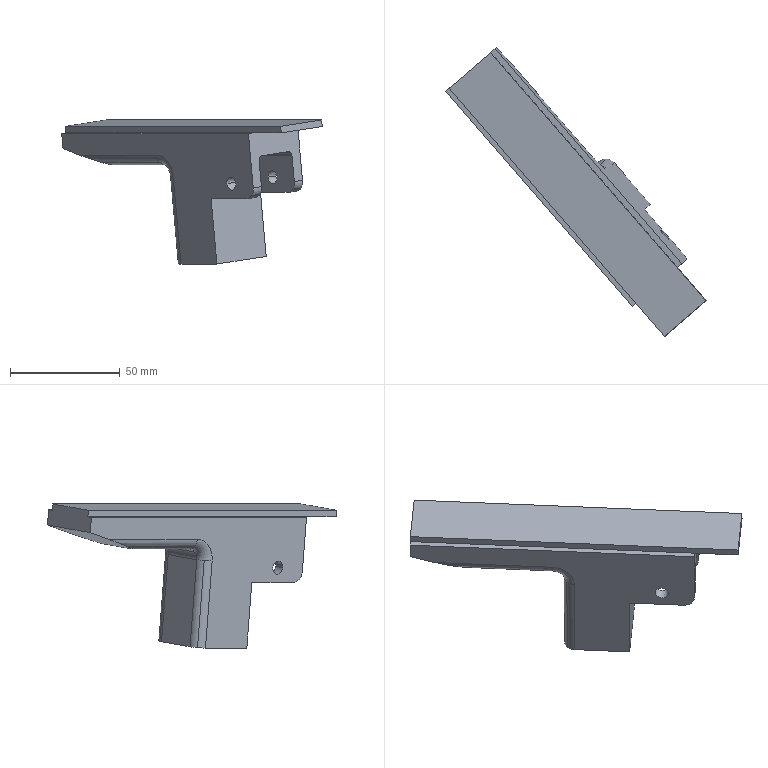Part | SolidWorks | features BaseBody 1 | 1 solid | 45 faces | box 118.942 x 131.952 x 65.78 mm | volume 109548 mm3 | cylinder 22 | plane 21 | torus 2 | commonest cylinder face diameters 10 x14 4 x4 6 x4
STEP:
#1=CARTESIAN_POINT('',(29.752,179.49,-230.441));
#2=VERTEX_POINT('',#1);
#3=CARTESIAN_POINT('',(33.684,174.958,-230.441));
#4=VERTEX_POINT('',#3);
#5=CARTESIAN_POINT('',(31.718,177.224,-230.441));
#6=DIRECTION('',(-0.7501,-0.6509,-0.1168));
#7=DIRECTION('',(0.6554,-0.7553,0.));
#8=AXIS2_PLACEMENT_3D('',#5,#6,#7);
#9=CIRCLE('',#8,3.);
#10=EDGE_CURVE('',#2,#4,#9,.T.);
#11=ORIENTED_EDGE('',*,*,#10,.F.);
#12=CARTESIAN_POINT('',(26.001,176.235,-231.025));
#13=VERTEX_POINT('',#12);
#14=CARTESIAN_POINT('',(48.504,195.763,-227.522));
#15=DIRECTION('',(-0.7501,-0.6509,-0.1168));
#16=VECTOR('',#15,1000.);
#17=LINE('',#14,#16);
#18=EDGE_CURVE('',#2,#13,#17,.T.);
#19=ORIENTED_EDGE('',*,*,#18,.T.);
#20=CARTESIAN_POINT('',(29.934,171.704,-231.025));
#21=VERTEX_POINT('',#20);
#22=CARTESIAN_POINT('',(27.968,173.969,-231.025));
#23=DIRECTION('',(0.7501,0.6509,0.1168));
#24=DIRECTION('',(0.6554,-0.7553,0.));
#25=AXIS2_PLACEMENT_3D('',#22,#23,#24);
#26=CIRCLE('',#25,3.);
#27=EDGE_CURVE('',#21,#13,#26,.T.);
#28=ORIENTED_EDGE('',*,*,#27,.F.);
#29=CARTESIAN_POINT('',(52.437,191.232,-227.522));
#30=DIRECTION('',(-0.7501,-0.6509,-0.1168));
#31=VECTOR('',#30,1000.);
#32=LINE('',#29,#31);
#33=EDGE_CURVE('',#4,#21,#32,.T.);
#34=ORIENTED_EDGE('',*,*,#33,.F.);
#35=EDGE_LOOP('',(#11,#19,#28,#34));
#36=FACE_OUTER_BOUND('',#35,.T.);
#37=CARTESIAN_POINT('',(50.47,193.498,-227.522));
#38=DIRECTION('',(-0.7501,-0.6509,-0.1168));
#39=DIRECTION('',(0.6554,-0.7553,0.));
#40=AXIS2_PLACEMENT_3D('',#37,#38,#39);
#41=CYLINDRICAL_SURFACE('',#40,3.);
#42=ADVANCED_FACE('',(#36),#41,.F.);
#43=CARTESIAN_POINT('',(48.504,195.763,-227.522));
#44=VERTEX_POINT('',#43);
#45=CARTESIAN_POINT('',(52.437,191.232,-227.522));
#46=VERTEX_POINT('',#45);
#47=CARTESIAN_POINT('',(50.47,193.498,-227.522));
#48=DIRECTION('',(-0.7501,-0.6509,-0.1168));
#49=DIRECTION('',(0.6554,-0.7553,0.));
#50=AXIS2_PLACEMENT_3D('',#47,#48,#49);
#51=CIRCLE('',#50,3.);
#52=EDGE_CURVE('',#44,#46,#51,.T.);
#53=ORIENTED_EDGE('',*,*,#52,.F.);
#54=CARTESIAN_POINT('',(44.754,192.509,-228.106));
#55=VERTEX_POINT('',#54);
#56=CARTESIAN_POINT('',(48.504,195.763,-227.522));
#57=DIRECTION('',(-0.7501,-0.6509,-0.1168));
#58=VECTOR('',#57,1000.);
#59=LINE('',#56,#58);
#60=EDGE_CURVE('',#44,#55,#59,.T.);
#61=ORIENTED_EDGE('',*,*,#60,.T.);
#62=CARTESIAN_POINT('',(48.686,187.977,-228.106));
#63=VERTEX_POINT('',#62);
#64=CARTESIAN_POINT('',(46.72,190.243,-228.106));
#65=DIRECTION('',(0.7501,0.6509,0.1168));
#66=DIRECTION('',(0.6554,-0.7553,0.));
#67=AXIS2_PLACEMENT_3D('',#64,#65,#66);
#68=CIRCLE('',#67,3.);
#69=EDGE_CURVE('',#63,#55,#68,.T.);
#70=ORIENTED_EDGE('',*,*,#69,.F.);
#71=CARTESIAN_POINT('',(52.437,191.232,-227.522));
#72=DIRECTION('',(-0.7501,-0.6509,-0.1168));
#73=VECTOR('',#72,1000.);
#74=LINE('',#71,#73);
#75=EDGE_CURVE('',#46,#63,#74,.T.);
#76=ORIENTED_EDGE('',*,*,#75,.F.);
#77=EDGE_LOOP('',(#53,#61,#70,#76));
#78=FACE_OUTER_BOUND('',#77,.T.);
#79=CARTESIAN_POINT('',(50.47,193.498,-227.522));
#80=DIRECTION('',(-0.7501,-0.6509,-0.1168));
#81=DIRECTION('',(0.6554,-0.7553,0.));
#82=AXIS2_PLACEMENT_3D('',#79,#80,#81);
#83=CYLINDRICAL_SURFACE('',#82,3.);
#84=ADVANCED_FACE('',(#78),#83,.F.);
#85=CARTESIAN_POINT('',(-41.121,251.264,-218.114));
#86=VERTEX_POINT('',#85);
#87=CARTESIAN_POINT('',(-31.062,242.523,-221.454));
#88=VERTEX_POINT('',#87);
#89=CARTESIAN_POINT('',(-41.121,251.264,-218.114));
#90=CARTESIAN_POINT('',(-37.715,247.58,-219.449));
#91=CARTESIAN_POINT('',(-34.183,244.51,-220.622));
#92=CARTESIAN_POINT('',(-31.062,242.523,-221.454));
#93=(BOUNDED_CURVE()B_SPLINE_CURVE(3,(#89,#90,#91,#92),.UNSPECIFIED.,.F.,.F.)B_SPLINE_CURVE_WITH_KNOTS((4,4),(4.712,5.498),.UNSPECIFIED.)CURVE()GEOMETRIC_REPRESENTATION_ITEM()RATIONAL_B_SPLINE_CURVE((1.,0.9493,0.9493,1.))REPRESENTATION_ITEM(''));
#94=EDGE_CURVE('',#86,#88,#93,.T.);
#95=ORIENTED_EDGE('',*,*,#94,.T.);
#96=CARTESIAN_POINT('',(-4.54,211.961,-221.454));
#97=VERTEX_POINT('',#96);
#98=CARTESIAN_POINT('',(-9.456,217.625,-221.454));
#99=DIRECTION('',(0.6554,-0.7553,0.));
#100=VECTOR('',#99,1000.);
#101=LINE('',#98,#100);
#102=EDGE_CURVE('',#88,#97,#101,.T.);
#103=ORIENTED_EDGE('',*,*,#102,.T.);
#104=CARTESIAN_POINT('',(-5.95,210.737,-218.114));
#105=VERTEX_POINT('',#104);
#106=CARTESIAN_POINT('',(-2.2,213.992,-217.53));
#107=DIRECTION('',(-0.6554,0.7553,0.));
#108=DIRECTION('',(0.0882,0.07654,-0.9932));
#109=AXIS2_PLACEMENT_3D('',#106,#107,#108);
#110=CIRCLE('',#109,5.);
#111=EDGE_CURVE('',#97,#105,#110,.T.);
#112=ORIENTED_EDGE('',*,*,#111,.T.);
#113=CARTESIAN_POINT('',(-10.866,216.402,-218.114));
#114=DIRECTION('',(-0.6554,0.7553,0.));
#115=VECTOR('',#114,1000.);
#116=LINE('',#113,#115);
#117=EDGE_CURVE('',#105,#86,#116,.T.);
#118=ORIENTED_EDGE('',*,*,#117,.T.);
#119=EDGE_LOOP('',(#95,#103,#112,#118));
#120=FACE_OUTER_BOUND('',#119,.T.);
#121=CARTESIAN_POINT('',(-7.116,219.656,-217.53));
#122=DIRECTION('',(0.6554,-0.7553,0.));
#123=DIRECTION('',(-0.468,-0.4062,-0.7848));
#124=AXIS2_PLACEMENT_3D('',#121,#122,#123);
#125=CYLINDRICAL_SURFACE('',#124,5.);
#126=ADVANCED_FACE('',(#120),#125,.T.);
#127=CARTESIAN_POINT('',(0.2672,207.573,-227.875));
#128=VERTEX_POINT('',#127);
#129=CARTESIAN_POINT('',(1.486,203.95,-228.046));
#130=VERTEX_POINT('',#129);
#131=CARTESIAN_POINT('',(5.236,207.205,-227.462));
#132=DIRECTION('',(-0.0882,-0.07654,0.9932));
#133=DIRECTION('',(-0.6554,0.7553,0.));
#134=AXIS2_PLACEMENT_3D('',#131,#132,#133);
#135=CIRCLE('',#134,5.);
#136=EDGE_CURVE('',#128,#130,#135,.T.);
#137=ORIENTED_EDGE('',*,*,#136,.F.);
#138=CARTESIAN_POINT('',(3.795,210.635,-267.601));
#139=VERTEX_POINT('',#138);
#140=CARTESIAN_POINT('',(-0.1738,207.191,-222.909));
#141=DIRECTION('',(0.0882,0.07654,-0.9932));
#142=VECTOR('',#141,1000.);
#143=LINE('',#140,#142);
#144=EDGE_CURVE('',#128,#139,#143,.T.);
#145=ORIENTED_EDGE('',*,*,#144,.T.);
#146=CARTESIAN_POINT('',(5.014,207.011,-267.772));
#147=VERTEX_POINT('',#146);
#148=CARTESIAN_POINT('',(8.764,210.266,-267.188));
#149=DIRECTION('',(-0.0882,-0.07654,0.9932));
#150=DIRECTION('',(-0.9939,0.07376,-0.08257));
#151=AXIS2_PLACEMENT_3D('',#148,#149,#150);
#152=CIRCLE('',#151,5.);
#153=EDGE_CURVE('',#139,#147,#152,.T.);
#154=ORIENTED_EDGE('',*,*,#153,.T.);
#155=CARTESIAN_POINT('',(1.045,203.567,-223.08));
#156=DIRECTION('',(-0.0882,-0.07654,0.9932));
#157=VECTOR('',#156,1000.);
#158=LINE('',#155,#157);
#159=EDGE_CURVE('',#147,#130,#158,.T.);
#160=ORIENTED_EDGE('',*,*,#159,.T.);
#161=EDGE_LOOP('',(#137,#145,#154,#160));
#162=FACE_OUTER_BOUND('',#161,.T.);
#163=CARTESIAN_POINT('',(4.795,206.822,-222.496));
#164=DIRECTION('',(0.0882,0.07654,-0.9932));
#165=DIRECTION('',(-0.9939,0.07376,-0.08257));
#166=AXIS2_PLACEMENT_3D('',#163,#164,#165);
#167=CYLINDRICAL_SURFACE('',#166,5.);
#168=ADVANCED_FACE('',(#162),#167,.T.);
#169=CARTESIAN_POINT('',(15.689,224.835,-221.615));
#170=VERTEX_POINT('',#169);
#171=CARTESIAN_POINT('',(13.243,227.393,-220.16));
#172=VERTEX_POINT('',#171);
#173=CARTESIAN_POINT('',(13.684,227.776,-225.126));
#174=DIRECTION('',(-0.7501,-0.6509,-0.1168));
#175=DIRECTION('',(0.4011,-0.5882,0.7023));
#176=AXIS2_PLACEMENT_3D('',#173,#174,#175);
#177=CIRCLE('',#176,5.);
#178=EDGE_CURVE('',#170,#172,#177,.T.);
#179=ORIENTED_EDGE('',*,*,#178,.F.);
#180=CARTESIAN_POINT('',(0.6876,211.816,-223.95));
#181=VERTEX_POINT('',#180);
#182=CARTESIAN_POINT('',(19.44,228.09,-221.031));
#183=DIRECTION('',(-0.7501,-0.6509,-0.1168));
#184=VECTOR('',#183,1000.);
#185=LINE('',#182,#184);
#186=EDGE_CURVE('',#170,#181,#185,.T.);
#187=ORIENTED_EDGE('',*,*,#186,.T.);
#188=CARTESIAN_POINT('',(-1.759,214.375,-222.496));
#189=VERTEX_POINT('',#188);
#190=CARTESIAN_POINT('',(-1.318,214.757,-227.462));
#191=DIRECTION('',(0.7501,0.6509,0.1168));
#192=DIRECTION('',(0.4011,-0.5882,0.7023));
#193=AXIS2_PLACEMENT_3D('',#190,#191,#192);
#194=CIRCLE('',#193,5.);
#195=EDGE_CURVE('',#189,#181,#194,.T.);
#196=ORIENTED_EDGE('',*,*,#195,.F.);
#197=CARTESIAN_POINT('',(16.993,230.648,-219.577));
#198=DIRECTION('',(0.7501,0.6509,0.1168));
#199=VECTOR('',#198,1000.);
#200=LINE('',#197,#199);
#201=EDGE_CURVE('',#189,#172,#200,.T.);
#202=ORIENTED_EDGE('',*,*,#201,.T.);
#203=EDGE_LOOP('',(#179,#187,#196,#202));
#204=FACE_OUTER_BOUND('',#203,.T.);
#205=CARTESIAN_POINT('',(17.434,231.031,-224.542));
#206=DIRECTION('',(-0.7501,-0.6509,-0.1168));
#207=DIRECTION('',(0.4011,-0.5882,0.7023));
#208=AXIS2_PLACEMENT_3D('',#205,#206,#207);
#209=CYLINDRICAL_SURFACE('',#208,5.);
#210=ADVANCED_FACE('',(#204),#209,.F.);
#211=CARTESIAN_POINT('',(-9.697,253.827,-220.16));
#212=VERTEX_POINT('',#211);
#213=CARTESIAN_POINT('',(-10.756,260.145,-218.293));
#214=VERTEX_POINT('',#213);
#215=CARTESIAN_POINT('',(-9.697,253.827,-220.16));
#216=CARTESIAN_POINT('',(-8.689,254.702,-220.004));
#217=CARTESIAN_POINT('',(-9.061,256.92,-219.348));
#218=CARTESIAN_POINT('',(-10.756,260.145,-218.293));
#219=(BOUNDED_CURVE()B_SPLINE_CURVE(3,(#215,#216,#217,#218),.UNSPECIFIED.,.F.,.F.)B_SPLINE_CURVE_WITH_KNOTS((4,4),(0.,0.7854),.UNSPECIFIED.)CURVE()GEOMETRIC_REPRESENTATION_ITEM()RATIONAL_B_SPLINE_CURVE((1.,0.9493,0.9493,1.))REPRESENTATION_ITEM(''));
#220=EDGE_CURVE('',#212,#214,#219,.T.);
#221=ORIENTED_EDGE('',*,*,#220,.T.);
#222=CARTESIAN_POINT('',(15.766,229.583,-218.293));
#223=VERTEX_POINT('',#222);
#224=CARTESIAN_POINT('',(10.85,235.247,-218.293));
#225=DIRECTION('',(0.6554,-0.7553,0.));
#226=VECTOR('',#225,1000.);
#227=LINE('',#224,#226);
#228=EDGE_CURVE('',#214,#223,#227,.T.);
#229=ORIENTED_EDGE('',*,*,#228,.T.);
#230=CARTESIAN_POINT('',(12.802,227.011,-215.195));
#231=DIRECTION('',(-0.6554,0.7553,0.));
#232=DIRECTION('',(0.7501,0.6509,0.1168));
#233=AXIS2_PLACEMENT_3D('',#230,#231,#232);
#234=CIRCLE('',#233,5.);
#235=EDGE_CURVE('',#223,#172,#234,.T.);
#236=ORIENTED_EDGE('',*,*,#235,.T.);
#237=CARTESIAN_POINT('',(8.327,233.058,-220.16));
#238=DIRECTION('',(-0.6554,0.7553,0.));
#239=VECTOR('',#238,1000.);
#240=LINE('',#237,#239);
#241=EDGE_CURVE('',#172,#212,#240,.T.);
#242=ORIENTED_EDGE('',*,*,#241,.T.);
#243=EDGE_LOOP('',(#221,#229,#236,#242));
#244=FACE_OUTER_BOUND('',#243,.T.);
#245=CARTESIAN_POINT('',(7.886,232.675,-215.195));
#246=DIRECTION('',(0.6554,-0.7553,0.));
#247=DIRECTION('',(0.5928,0.5144,-0.6197));
#248=AXIS2_PLACEMENT_3D('',#245,#246,#247);
#249=CYLINDRICAL_SURFACE('',#248,5.);
#250=ADVANCED_FACE('',(#244),#249,.T.);
#251=CARTESIAN_POINT('',(20.573,225.195,-224.713));
#252=VERTEX_POINT('',#251);
#253=CARTESIAN_POINT('',(16.961,224.,-225.126));
#254=VERTEX_POINT('',#253);
#255=CARTESIAN_POINT('',(20.238,220.224,-225.126));
#256=DIRECTION('',(-0.0882,-0.07654,0.9932));
#257=DIRECTION('',(0.7501,0.6509,0.1168));
#258=AXIS2_PLACEMENT_3D('',#255,#256,#257);
#259=CIRCLE('',#258,5.);
#260=EDGE_CURVE('',#252,#254,#259,.T.);
#261=ORIENTED_EDGE('',*,*,#260,.F.);
#262=CARTESIAN_POINT('',(24.101,228.257,-264.44));
#263=VERTEX_POINT('',#262);
#264=CARTESIAN_POINT('',(20.132,224.813,-219.748));
#265=DIRECTION('',(0.0882,0.07654,-0.9932));
#266=VECTOR('',#265,1000.);
#267=LINE('',#264,#266);
#268=EDGE_CURVE('',#252,#263,#267,.T.);
#269=ORIENTED_EDGE('',*,*,#268,.T.);
#270=CARTESIAN_POINT('',(20.489,227.061,-264.853));
#271=VERTEX_POINT('',#270);
#272=CARTESIAN_POINT('',(23.766,223.285,-264.853));
#273=DIRECTION('',(-0.0882,-0.07654,0.9932));
#274=DIRECTION('',(0.06694,0.9943,0.08257));
#275=AXIS2_PLACEMENT_3D('',#272,#273,#274);
#276=CIRCLE('',#275,5.);
#277=EDGE_CURVE('',#263,#271,#276,.T.);
#278=ORIENTED_EDGE('',*,*,#277,.T.);
#279=CARTESIAN_POINT('',(16.52,223.617,-220.16));
#280=DIRECTION('',(-0.0882,-0.07654,0.9932));
#281=VECTOR('',#280,1000.);
#282=LINE('',#279,#281);
#283=EDGE_CURVE('',#271,#254,#282,.T.);
#284=ORIENTED_EDGE('',*,*,#283,.T.);
#285=EDGE_LOOP('',(#261,#269,#278,#284));
#286=FACE_OUTER_BOUND('',#285,.T.);
#287=CARTESIAN_POINT('',(19.797,219.841,-220.16));
#288=DIRECTION('',(0.0882,0.07654,-0.9932));
#289=DIRECTION('',(0.06694,0.9943,0.08257));
#290=AXIS2_PLACEMENT_3D('',#287,#288,#289);
#291=CYLINDRICAL_SURFACE('',#290,5.);
#292=ADVANCED_FACE('',(#286),#291,.T.);
#293=CARTESIAN_POINT('',(55.669,178.149,-218.174));
#294=VERTEX_POINT('',#293);
#295=CARTESIAN_POINT('',(55.105,177.659,-216.838));
#296=VERTEX_POINT('',#295);
#297=CARTESIAN_POINT('',(54.169,176.847,-218.408));
#298=DIRECTION('',(0.6554,-0.7553,0.));
#299=DIRECTION('',(0.468,0.4062,0.7848));
#300=AXIS2_PLACEMENT_3D('',#297,#298,#299);
#301=CIRCLE('',#300,2.);
#302=EDGE_CURVE('',#294,#296,#301,.T.);
#303=ORIENTED_EDGE('',*,*,#302,.T.);
#304=CARTESIAN_POINT('',(38.72,196.541,-216.838));
#305=VERTEX_POINT('',#304);
#306=CARTESIAN_POINT('',(55.105,177.659,-216.838));
#307=DIRECTION('',(-0.6554,0.7553,0.));
#308=VECTOR('',#307,1000.);
#309=LINE('',#306,#308);
#310=EDGE_CURVE('',#296,#305,#309,.T.);
#311=ORIENTED_EDGE('',*,*,#310,.T.);
#312=CARTESIAN_POINT('',(39.284,197.03,-218.174));
#313=VERTEX_POINT('',#312);
#314=CARTESIAN_POINT('',(37.784,195.728,-218.408));
#315=DIRECTION('',(0.6554,-0.7553,0.));
#316=DIRECTION('',(0.468,0.4062,0.7848));
#317=AXIS2_PLACEMENT_3D('',#314,#315,#316);
#318=CIRCLE('',#317,2.);
#319=EDGE_CURVE('',#313,#305,#318,.T.);
#320=ORIENTED_EDGE('',*,*,#319,.F.);
#321=CARTESIAN_POINT('',(55.669,178.149,-218.174));
#322=DIRECTION('',(0.6554,-0.7553,0.));
#323=VECTOR('',#322,1000.);
#324=LINE('',#321,#323);
#325=EDGE_CURVE('',#313,#294,#324,.T.);
#326=ORIENTED_EDGE('',*,*,#325,.T.);
#327=EDGE_LOOP('',(#303,#311,#320,#326));
#328=FACE_OUTER_BOUND('',#327,.T.);
#329=CARTESIAN_POINT('',(54.169,176.847,-218.408));
#330=DIRECTION('',(-0.6554,0.7553,0.));
#331=DIRECTION('',(0.468,0.4062,0.7848));
#332=AXIS2_PLACEMENT_3D('',#329,#330,#331);
#333=CYLINDRICAL_SURFACE('',#332,2.);
#334=ADVANCED_FACE('',(#328),#333,.F.);
#335=CARTESIAN_POINT('',(41.991,166.279,-218.29));
#336=VERTEX_POINT('',#335);
#337=CARTESIAN_POINT('',(40.982,165.403,-219.037));
#338=VERTEX_POINT('',#337);
#339=CARTESIAN_POINT('',(42.168,166.432,-220.276));
#340=DIRECTION('',(0.6554,-0.7553,0.));
#341=DIRECTION('',(-0.5928,-0.5144,0.6197));
#342=AXIS2_PLACEMENT_3D('',#339,#340,#341);
#343=CIRCLE('',#342,2.);
#344=EDGE_CURVE('',#336,#338,#343,.T.);
#345=ORIENTED_EDGE('',*,*,#344,.T.);
#346=CARTESIAN_POINT('',(24.597,184.284,-219.037));
#347=VERTEX_POINT('',#346);
#348=CARTESIAN_POINT('',(40.982,165.403,-219.037));
#349=DIRECTION('',(-0.6554,0.7553,0.));
#350=VECTOR('',#349,1000.);
#351=LINE('',#348,#350);
#352=EDGE_CURVE('',#338,#347,#351,.T.);
#353=ORIENTED_EDGE('',*,*,#352,.T.);
#354=CARTESIAN_POINT('',(25.606,185.16,-218.29));
#355=VERTEX_POINT('',#354);
#356=CARTESIAN_POINT('',(25.782,185.313,-220.276));
#357=DIRECTION('',(0.6554,-0.7553,0.));
#358=DIRECTION('',(-0.5928,-0.5144,0.6197));
#359=AXIS2_PLACEMENT_3D('',#356,#357,#358);
#360=CIRCLE('',#359,2.);
#361=EDGE_CURVE('',#355,#347,#360,.T.);
#362=ORIENTED_EDGE('',*,*,#361,.F.);
#363=CARTESIAN_POINT('',(41.991,166.279,-218.29));
#364=DIRECTION('',(0.6554,-0.7553,0.));
#365=VECTOR('',#364,1000.);
#366=LINE('',#363,#365);
#367=EDGE_CURVE('',#355,#336,#366,.T.);
#368=ORIENTED_EDGE('',*,*,#367,.T.);
#369=EDGE_LOOP('',(#345,#353,#362,#368));
#370=FACE_OUTER_BOUND('',#369,.T.);
#371=CARTESIAN_POINT('',(42.168,166.432,-220.276));
#372=DIRECTION('',(-0.6554,0.7553,0.));
#373=DIRECTION('',(-0.5928,-0.5144,0.6197));
#374=AXIS2_PLACEMENT_3D('',#371,#372,#373);
#375=CYLINDRICAL_SURFACE('',#374,2.);
#376=ADVANCED_FACE('',(#370),#375,.F.);
#377=CARTESIAN_POINT('',(37.976,162.794,-233.011));
#378=VERTEX_POINT('',#377);
#379=CARTESIAN_POINT('',(37.328,164.17,-236.523));
#380=VERTEX_POINT('',#379);
#381=CARTESIAN_POINT('',(34.698,166.57,-233.011));
#382=DIRECTION('',(0.7501,0.6509,0.1168));
#383=DIRECTION('',(0.5258,-0.4799,-0.7023));
#384=AXIS2_PLACEMENT_3D('',#381,#382,#383);
#385=CIRCLE('',#384,5.);
#386=EDGE_CURVE('',#378,#380,#385,.T.);
#387=ORIENTED_EDGE('',*,*,#386,.T.);
#388=CARTESIAN_POINT('',(41.078,167.425,-235.939));
#389=VERTEX_POINT('',#388);
#390=CARTESIAN_POINT('',(37.328,164.17,-236.523));
#391=DIRECTION('',(0.7501,0.6509,0.1168));
#392=VECTOR('',#391,1000.);
#393=LINE('',#390,#392);
#394=EDGE_CURVE('',#380,#389,#393,.T.);
#395=ORIENTED_EDGE('',*,*,#394,.T.);
#396=CARTESIAN_POINT('',(41.726,166.048,-232.428));
#397=VERTEX_POINT('',#396);
#398=CARTESIAN_POINT('',(38.449,169.825,-232.428));
#399=DIRECTION('',(-0.7501,-0.6509,-0.1168));
#400=DIRECTION('',(0.5258,-0.4799,-0.7023));
#401=AXIS2_PLACEMENT_3D('',#398,#399,#400);
#402=CIRCLE('',#401,5.);
#403=EDGE_CURVE('',#389,#397,#402,.T.);
#404=ORIENTED_EDGE('',*,*,#403,.T.);
#405=CARTESIAN_POINT('',(37.976,162.794,-233.011));
#406=DIRECTION('',(-0.7501,-0.6509,-0.1168));
#407=VECTOR('',#406,1000.);
#408=LINE('',#405,#407);
#409=EDGE_CURVE('',#397,#378,#408,.T.);
#410=ORIENTED_EDGE('',*,*,#409,.T.);
#411=EDGE_LOOP('',(#387,#395,#404,#410));
#412=FACE_OUTER_BOUND('',#411,.T.);
#413=CARTESIAN_POINT('',(34.698,166.57,-233.011));
#414=DIRECTION('',(0.7501,0.6509,0.1168));
#415=DIRECTION('',(0.5258,-0.4799,-0.7023));
#416=AXIS2_PLACEMENT_3D('',#413,#414,#415);
#417=CYLINDRICAL_SURFACE('',#416,5.);
#418=ADVANCED_FACE('',(#412),#417,.T.);
#419=CARTESIAN_POINT('',(56.728,179.067,-230.092));
#420=VERTEX_POINT('',#419);
#421=CARTESIAN_POINT('',(56.08,180.444,-233.603));
#422=VERTEX_POINT('',#421);
#423=CARTESIAN_POINT('',(53.451,182.843,-230.092));
#424=DIRECTION('',(0.7501,0.6509,0.1168));
#425=DIRECTION('',(0.5258,-0.4799,-0.7023));
#426=AXIS2_PLACEMENT_3D('',#423,#424,#425);
#427=CIRCLE('',#426,5.);
#428=EDGE_CURVE('',#420,#422,#427,.T.);
#429=ORIENTED_EDGE('',*,*,#428,.T.);
#430=CARTESIAN_POINT('',(59.83,183.698,-233.02));
#431=VERTEX_POINT('',#430);
#432=CARTESIAN_POINT('',(37.328,164.17,-236.523));
#433=DIRECTION('',(0.7501,0.6509,0.1168));
#434=VECTOR('',#433,1000.);
#435=LINE('',#432,#434);
#436=EDGE_CURVE('',#422,#431,#435,.T.);
#437=ORIENTED_EDGE('',*,*,#436,.T.);
#438=CARTESIAN_POINT('',(60.478,182.322,-229.508));
#439=VERTEX_POINT('',#438);
#440=CARTESIAN_POINT('',(57.201,186.098,-229.508));
#441=DIRECTION('',(-0.7501,-0.6509,-0.1168));
#442=DIRECTION('',(0.5258,-0.4799,-0.7023));
#443=AXIS2_PLACEMENT_3D('',#440,#441,#442);
#444=CIRCLE('',#443,5.);
#445=EDGE_CURVE('',#431,#439,#444,.T.);
#446=ORIENTED_EDGE('',*,*,#445,.T.);
#447=CARTESIAN_POINT('',(37.976,162.794,-233.011));
#448=DIRECTION('',(-0.7501,-0.6509,-0.1168));
#449=VECTOR('',#448,1000.);
#450=LINE('',#447,#449);
#451=EDGE_CURVE('',#439,#420,#450,.T.);
#452=ORIENTED_EDGE('',*,*,#451,.T.);
#453=EDGE_LOOP('',(#429,#437,#446,#452));
#454=FACE_OUTER_BOUND('',#453,.T.);
#455=CARTESIAN_POINT('',(34.698,166.57,-233.011));
#456=DIRECTION('',(0.7501,0.6509,0.1168));
#457=DIRECTION('',(0.5258,-0.4799,-0.7023));
#458=AXIS2_PLACEMENT_3D('',#455,#456,#457);
#459=CYLINDRICAL_SURFACE('',#458,5.);
#460=ADVANCED_FACE('',(#454),#459,.T.);
#461=ORIENTED_EDGE('',*,*,#27,.T.);
#462=CARTESIAN_POINT('',(27.968,173.969,-231.025));
#463=DIRECTION('',(0.7501,0.6509,0.1168));
#464=DIRECTION('',(0.6554,-0.7553,0.));
#465=AXIS2_PLACEMENT_3D('',#462,#463,#464);
#466=CIRCLE('',#465,3.);
#467=EDGE_CURVE('',#13,#21,#466,.T.);
#468=ORIENTED_EDGE('',*,*,#467,.T.);
#469=EDGE_LOOP('',(#461,#468));
#470=FACE_BOUND('',#469,.T.);
#471=ORIENTED_EDGE('',*,*,#159,.F.);
#472=CARTESIAN_POINT('',(21.4,188.13,-267.772));
#473=VERTEX_POINT('',#472);
#474=CARTESIAN_POINT('',(1.737,210.788,-267.772));
#475=DIRECTION('',(0.6554,-0.7553,0.));
#476=VECTOR('',#475,1000.);
#477=LINE('',#474,#476);
#478=EDGE_CURVE('',#147,#473,#477,.T.);
#479=ORIENTED_EDGE('',*,*,#478,.T.);
#480=CARTESIAN_POINT('',(18.754,185.834,-237.977));
#481=VERTEX_POINT('',#480);
#482=CARTESIAN_POINT('',(21.4,188.13,-267.772));
#483=DIRECTION('',(-0.0882,-0.07654,0.9932));
#484=VECTOR('',#483,1000.);
#485=LINE('',#482,#484);
#486=EDGE_CURVE('',#473,#481,#485,.T.);
#487=ORIENTED_EDGE('',*,*,#486,.T.);
#488=CARTESIAN_POINT('',(35.139,166.952,-237.977));
#489=VERTEX_POINT('',#488);
#490=CARTESIAN_POINT('',(38.417,163.176,-237.977));
#491=DIRECTION('',(-0.6554,0.7553,0.));
#492=VECTOR('',#491,1000.);
#493=LINE('',#490,#492);
#494=EDGE_CURVE('',#489,#481,#493,.T.);
#495=ORIENTED_EDGE('',*,*,#494,.F.);
#496=CARTESIAN_POINT('',(34.698,166.57,-233.011));
#497=DIRECTION('',(0.7501,0.6509,0.1168));
#498=DIRECTION('',(0.5258,-0.4799,-0.7023));
#499=AXIS2_PLACEMENT_3D('',#496,#497,#498);
#500=CIRCLE('',#499,5.);
#501=EDGE_CURVE('',#380,#489,#500,.T.);
#502=ORIENTED_EDGE('',*,*,#501,.F.);
#503=ORIENTED_EDGE('',*,*,#386,.F.);
#504=CARTESIAN_POINT('',(35.771,160.88,-208.183));
#505=VERTEX_POINT('',#504);
#506=CARTESIAN_POINT('',(35.771,160.88,-208.183));
#507=DIRECTION('',(0.0882,0.07654,-0.9932));
#508=VECTOR('',#507,1000.);
#509=LINE('',#506,#508);
#510=EDGE_CURVE('',#505,#378,#509,.T.);
#511=ORIENTED_EDGE('',*,*,#510,.F.);
#512=CARTESIAN_POINT('',(-49.435,259.063,-208.183));
#513=VERTEX_POINT('',#512);
#514=CARTESIAN_POINT('',(16.108,183.538,-208.183));
#515=DIRECTION('',(-0.6554,0.7553,0.));
#516=VECTOR('',#515,1000.);
#517=LINE('',#514,#516);
#518=EDGE_CURVE('',#505,#513,#517,.T.);
#519=ORIENTED_EDGE('',*,*,#518,.T.);
#520=CARTESIAN_POINT('',(-48.821,259.596,-215.096));
#521=VERTEX_POINT('',#520);
#522=CARTESIAN_POINT('',(-49.435,259.063,-208.183));
#523=DIRECTION('',(0.0882,0.07654,-0.9932));
#524=VECTOR('',#523,1000.);
#525=LINE('',#522,#524);
#526=EDGE_CURVE('',#513,#521,#525,.T.);
#527=ORIENTED_EDGE('',*,*,#526,.T.);
#528=CARTESIAN_POINT('',(-6.615,213.929,-231.636));
#529=DIRECTION('',(-0.6559,0.7097,0.257));
#530=VECTOR('',#529,1000.);
#531=LINE('',#528,#530);
#532=EDGE_CURVE('',#86,#521,#531,.T.);
#533=ORIENTED_EDGE('',*,*,#532,.F.);
#534=ORIENTED_EDGE('',*,*,#117,.F.);
#535=CARTESIAN_POINT('',(-5.068,211.503,-228.046));
#536=DIRECTION('',(-0.7501,-0.6509,-0.1168));
#537=DIRECTION('',(0.4011,-0.5882,0.7023));
#538=AXIS2_PLACEMENT_3D('',#535,#536,#537);
#539=CIRCLE('',#538,10.);
#540=EDGE_CURVE('',#130,#105,#539,.T.);
#541=ORIENTED_EDGE('',*,*,#540,.F.);
#542=EDGE_LOOP('',(#471,#479,#487,#495,#502,#503,#511,#519,#527,#533,#534,#541));
#543=FACE_OUTER_BOUND('',#542,.T.);
#544=CARTESIAN_POINT('',(27.262,173.357,-223.08));
#545=DIRECTION('',(0.7501,0.6509,0.1168));
#546=DIRECTION('',(-0.6554,0.7553,0.));
#547=AXIS2_PLACEMENT_3D('',#544,#545,#546);
#548=PLANE('',#547);
#549=ADVANCED_FACE('',(#470,#543),#548,.F.);
#550=ORIENTED_EDGE('',*,*,#409,.F.);
#551=CARTESIAN_POINT('',(40.668,165.13,-220.51));
#552=VERTEX_POINT('',#551);
#553=CARTESIAN_POINT('',(40.997,165.415,-224.213));
#554=DIRECTION('',(-0.0882,-0.07654,0.9932));
#555=VECTOR('',#554,1000.);
#556=LINE('',#553,#555);
#557=EDGE_CURVE('',#397,#552,#556,.T.);
#558=ORIENTED_EDGE('',*,*,#557,.T.);
#559=CARTESIAN_POINT('',(42.168,166.432,-220.276));
#560=DIRECTION('',(0.6554,-0.7553,0.));
#561=DIRECTION('',(-0.5928,-0.5144,0.6197));
#562=AXIS2_PLACEMENT_3D('',#559,#560,#561);
#563=CIRCLE('',#562,2.);
#564=EDGE_CURVE('',#338,#552,#563,.T.);
#565=ORIENTED_EDGE('',*,*,#564,.F.);
#566=ORIENTED_EDGE('',*,*,#344,.F.);
#567=CARTESIAN_POINT('',(53.993,176.694,-216.421));
#568=VERTEX_POINT('',#567);
#569=CARTESIAN_POINT('',(38.616,163.349,-218.815));
#570=DIRECTION('',(0.7501,0.6509,0.1168));
#571=VECTOR('',#570,1000.);
#572=LINE('',#569,#571);
#573=EDGE_CURVE('',#336,#568,#572,.T.);
#574=ORIENTED_EDGE('',*,*,#573,.T.);
#575=CARTESIAN_POINT('',(54.169,176.847,-218.408));
#576=DIRECTION('',(0.6554,-0.7553,0.));
#577=DIRECTION('',(0.468,0.4062,0.7848));
#578=AXIS2_PLACEMENT_3D('',#575,#576,#577);
#579=CIRCLE('',#578,2.);
#580=EDGE_CURVE('',#296,#568,#579,.T.);
#581=ORIENTED_EDGE('',*,*,#580,.F.);
#582=ORIENTED_EDGE('',*,*,#302,.F.);
#583=CARTESIAN_POINT('',(55.008,177.575,-210.725));
#584=DIRECTION('',(0.0882,0.07654,-0.9932));
#585=VECTOR('',#584,1000.);
#586=LINE('',#583,#585);
#587=EDGE_CURVE('',#294,#420,#586,.T.);
#588=ORIENTED_EDGE('',*,*,#587,.T.);
#589=ORIENTED_EDGE('',*,*,#451,.F.);
#590=CARTESIAN_POINT('',(58.273,180.408,-204.679));
#591=VERTEX_POINT('',#590);
#592=CARTESIAN_POINT('',(58.273,180.408,-204.679));
#593=DIRECTION('',(0.0882,0.07654,-0.9932));
#594=VECTOR('',#593,1000.);
#595=LINE('',#592,#594);
#596=EDGE_CURVE('',#591,#439,#595,.T.);
#597=ORIENTED_EDGE('',*,*,#596,.F.);
#598=CARTESIAN_POINT('',(56.398,178.781,-204.971));
#599=VERTEX_POINT('',#598);
#600=CARTESIAN_POINT('',(35.771,160.88,-208.183));
#601=DIRECTION('',(0.7501,0.6509,0.1168));
#602=VECTOR('',#601,1000.);
#603=LINE('',#600,#602);
#604=EDGE_CURVE('',#599,#591,#603,.T.);
#605=ORIENTED_EDGE('',*,*,#604,.F.);
#606=CARTESIAN_POINT('',(37.646,162.507,-207.891));
#607=VERTEX_POINT('',#606);
#608=CARTESIAN_POINT('',(35.771,160.88,-208.183));
#609=DIRECTION('',(0.7501,0.6509,0.1168));
#610=VECTOR('',#609,1000.);
#611=LINE('',#608,#610);
#612=EDGE_CURVE('',#607,#599,#611,.T.);
#613=ORIENTED_EDGE('',*,*,#612,.F.);
#614=CARTESIAN_POINT('',(35.771,160.88,-208.183));
#615=DIRECTION('',(0.7501,0.6509,0.1168));
#616=VECTOR('',#615,1000.);
#617=LINE('',#614,#616);
#618=EDGE_CURVE('',#505,#607,#617,.T.);
#619=ORIENTED_EDGE('',*,*,#618,.F.);
#620=ORIENTED_EDGE('',*,*,#510,.T.);
#621=EDGE_LOOP('',(#550,#558,#565,#566,#574,#581,#582,#588,#589,#597,#605,#613,#619,#620));
#622=FACE_OUTER_BOUND('',#621,.T.);
#623=CARTESIAN_POINT('',(35.771,160.88,-208.183));
#624=DIRECTION('',(0.6554,-0.7553,0.));
#625=DIRECTION('',(-0.0882,-0.07654,0.9932));
#626=AXIS2_PLACEMENT_3D('',#623,#624,#625);
#627=PLANE('',#626);
#628=ADVANCED_FACE('',(#622),#627,.T.);
#629=CARTESIAN_POINT('',(37.607,195.575,-216.421));
#630=VERTEX_POINT('',#629);
#631=CARTESIAN_POINT('',(53.993,176.694,-216.421));
#632=DIRECTION('',(-0.6554,0.7553,0.));
#633=VECTOR('',#632,1000.);
#634=LINE('',#631,#633);
#635=EDGE_CURVE('',#568,#630,#634,.T.);
#636=ORIENTED_EDGE('',*,*,#635,.F.);
#637=ORIENTED_EDGE('',*,*,#573,.F.);
#638=ORIENTED_EDGE('',*,*,#367,.F.);
#639=CARTESIAN_POINT('',(24.106,183.858,-218.523));
#640=DIRECTION('',(0.7501,0.6509,0.1168));
#641=VECTOR('',#640,1000.);
#642=LINE('',#639,#641);
#643=EDGE_CURVE('',#355,#630,#642,.T.);
#644=ORIENTED_EDGE('',*,*,#643,.T.);
#645=EDGE_LOOP('',(#636,#637,#638,#644));
#646=FACE_OUTER_BOUND('',#645,.T.);
#647=CARTESIAN_POINT('',(40.491,164.977,-218.523));
#648=DIRECTION('',(-0.0882,-0.07654,0.9932));
#649=DIRECTION('',(-0.6554,0.7553,0.));
#650=AXIS2_PLACEMENT_3D('',#647,#648,#649);
#651=PLANE('',#650);
#652=ADVANCED_FACE('',(#646),#651,.F.);
#653=ORIENTED_EDGE('',*,*,#436,.F.);
#654=CARTESIAN_POINT('',(53.892,183.226,-235.058));
#655=VERTEX_POINT('',#654);
#656=CARTESIAN_POINT('',(53.451,182.843,-230.092));
#657=DIRECTION('',(0.7501,0.6509,0.1168));
#658=DIRECTION('',(0.5258,-0.4799,-0.7023));
#659=AXIS2_PLACEMENT_3D('',#656,#657,#658);
#660=CIRCLE('',#659,5.);
#661=EDGE_CURVE('',#422,#655,#660,.T.);
#662=ORIENTED_EDGE('',*,*,#661,.T.);
#663=CARTESIAN_POINT('',(57.642,186.481,-234.474));
#664=VERTEX_POINT('',#663);
#665=CARTESIAN_POINT('',(35.139,166.952,-237.977));
#666=DIRECTION('',(0.7501,0.6509,0.1168));
#667=VECTOR('',#666,1000.);
#668=LINE('',#665,#667);
#669=EDGE_CURVE('',#655,#664,#668,.T.);
#670=ORIENTED_EDGE('',*,*,#669,.T.);
#671=CARTESIAN_POINT('',(57.201,186.098,-229.508));
#672=DIRECTION('',(-0.7501,-0.6509,-0.1168));
#673=DIRECTION('',(0.5258,-0.4799,-0.7023));
#674=AXIS2_PLACEMENT_3D('',#671,#672,#673);
#675=CIRCLE('',#674,5.);
#676=EDGE_CURVE('',#664,#431,#675,.T.);
#677=ORIENTED_EDGE('',*,*,#676,.T.);
#678=EDGE_LOOP('',(#653,#662,#670,#677));
#679=FACE_OUTER_BOUND('',#678,.T.);
#680=CARTESIAN_POINT('',(34.698,166.57,-233.011));
#681=DIRECTION('',(0.7501,0.6509,0.1168));
#682=DIRECTION('',(0.5258,-0.4799,-0.7023));
#683=AXIS2_PLACEMENT_3D('',#680,#681,#682);
#684=CYLINDRICAL_SURFACE('',#683,5.);
#685=ADVANCED_FACE('',(#679),#684,.T.);
#686=CARTESIAN_POINT('',(38.89,170.207,-237.393));
#687=VERTEX_POINT('',#686);
#688=CARTESIAN_POINT('',(35.139,166.952,-237.977));
#689=DIRECTION('',(0.7501,0.6509,0.1168));
#690=VECTOR('',#689,1000.);
#691=LINE('',#688,#690);
#692=EDGE_CURVE('',#489,#687,#691,.T.);
#693=ORIENTED_EDGE('',*,*,#692,.F.);
#694=ORIENTED_EDGE('',*,*,#494,.T.);
#695=CARTESIAN_POINT('',(41.256,205.362,-234.474));
#696=VERTEX_POINT('',#695);
#697=CARTESIAN_POINT('',(18.754,185.834,-237.977));
#698=DIRECTION('',(0.7501,0.6509,0.1168));
#699=VECTOR('',#698,1000.);
#700=LINE('',#697,#699);
#701=EDGE_CURVE('',#481,#696,#700,.T.);
#702=ORIENTED_EDGE('',*,*,#701,.T.);
#703=CARTESIAN_POINT('',(60.919,182.705,-234.474));
#704=DIRECTION('',(-0.6554,0.7553,0.));
#705=VECTOR('',#704,1000.);
#706=LINE('',#703,#705);
#707=EDGE_CURVE('',#664,#696,#706,.T.);
#708=ORIENTED_EDGE('',*,*,#707,.F.);
#709=ORIENTED_EDGE('',*,*,#669,.F.);
#710=CARTESIAN_POINT('',(40.783,198.331,-235.058));
#711=VERTEX_POINT('',#710);
#712=CARTESIAN_POINT('',(57.169,179.45,-235.058));
#713=DIRECTION('',(-0.6554,0.7553,0.));
#714=VECTOR('',#713,1000.);
#715=LINE('',#712,#714);
#716=EDGE_CURVE('',#655,#711,#715,.T.);
#717=ORIENTED_EDGE('',*,*,#716,.T.);
#718=CARTESIAN_POINT('',(25.781,185.312,-237.393));
#719=VERTEX_POINT('',#718);
#720=CARTESIAN_POINT('',(27.656,186.94,-237.101));
#721=DIRECTION('',(-0.7501,-0.6509,-0.1168));
#722=VECTOR('',#721,1000.);
#723=LINE('',#720,#722);
#724=EDGE_CURVE('',#711,#719,#723,.T.);
#725=ORIENTED_EDGE('',*,*,#724,.T.);
#726=CARTESIAN_POINT('',(42.167,166.431,-237.393));
#727=DIRECTION('',(0.6554,-0.7553,0.));
#728=VECTOR('',#727,1000.);
#729=LINE('',#726,#728);
#730=EDGE_CURVE('',#719,#687,#729,.T.);
#731=ORIENTED_EDGE('',*,*,#730,.T.);
#732=EDGE_LOOP('',(#693,#694,#702,#708,#709,#717,#725,#731));
#733=FACE_OUTER_BOUND('',#732,.T.);
#734=CARTESIAN_POINT('',(38.417,163.176,-237.977));
#735=DIRECTION('',(0.0882,0.07654,-0.9932));
#736=DIRECTION('',(-0.7501,-0.6509,-0.1168));
#737=AXIS2_PLACEMENT_3D('',#734,#735,#736);
#738=PLANE('',#737);
#739=ADVANCED_FACE('',(#733),#738,.T.);
#740=ORIENTED_EDGE('',*,*,#394,.F.);
#741=ORIENTED_EDGE('',*,*,#501,.T.);
#742=ORIENTED_EDGE('',*,*,#692,.T.);
#743=CARTESIAN_POINT('',(38.449,169.825,-232.428));
#744=DIRECTION('',(-0.7501,-0.6509,-0.1168));
#745=DIRECTION('',(0.5258,-0.4799,-0.7023));
#746=AXIS2_PLACEMENT_3D('',#743,#744,#745);
#747=CIRCLE('',#746,5.);
#748=EDGE_CURVE('',#687,#389,#747,.T.);
#749=ORIENTED_EDGE('',*,*,#748,.T.);
#750=EDGE_LOOP('',(#740,#741,#742,#749));
#751=FACE_OUTER_BOUND('',#750,.T.);
#752=CARTESIAN_POINT('',(34.698,166.57,-233.011));
#753=DIRECTION('',(0.7501,0.6509,0.1168));
#754=DIRECTION('',(0.5258,-0.4799,-0.7023));
#755=AXIS2_PLACEMENT_3D('',#752,#753,#754);
#756=CYLINDRICAL_SURFACE('',#755,5.);
#757=ADVANCED_FACE('',(#751),#756,.T.);
#758=CARTESIAN_POINT('',(31.718,177.224,-230.441));
#759=DIRECTION('',(-0.7501,-0.6509,-0.1168));
#760=DIRECTION('',(0.6554,-0.7553,0.));
#761=AXIS2_PLACEMENT_3D('',#758,#759,#760);
#762=CIRCLE('',#761,3.);
#763=EDGE_CURVE('',#4,#2,#762,.T.);
#764=ORIENTED_EDGE('',*,*,#763,.T.);
#765=ORIENTED_EDGE('',*,*,#10,.T.);
#766=EDGE_LOOP('',(#764,#765));
#767=FACE_BOUND('',#766,.T.);
#768=CARTESIAN_POINT('',(24.282,184.011,-220.51));
#769=VERTEX_POINT('',#768);
#770=CARTESIAN_POINT('',(40.668,165.13,-220.51));
#771=DIRECTION('',(-0.6554,0.7553,0.));
#772=VECTOR('',#771,1000.);
#773=LINE('',#770,#772);
#774=EDGE_CURVE('',#552,#769,#773,.T.);
#775=ORIENTED_EDGE('',*,*,#774,.F.);
#776=ORIENTED_EDGE('',*,*,#557,.F.);
#777=ORIENTED_EDGE('',*,*,#403,.F.);
#778=ORIENTED_EDGE('',*,*,#748,.F.);
#779=ORIENTED_EDGE('',*,*,#730,.F.);
#780=CARTESIAN_POINT('',(26.086,185.577,-240.827));
#781=DIRECTION('',(-0.0882,-0.07654,0.9932));
#782=VECTOR('',#781,1000.);
#783=LINE('',#780,#782);
#784=EDGE_CURVE('',#719,#769,#783,.T.);
#785=ORIENTED_EDGE('',*,*,#784,.T.);
#786=EDGE_LOOP('',(#775,#776,#777,#778,#779,#785));
#787=FACE_OUTER_BOUND('',#786,.T.);
#788=CARTESIAN_POINT('',(42.472,166.696,-240.827));
#789=DIRECTION('',(-0.7501,-0.6509,-0.1168));
#790=DIRECTION('',(0.0882,0.07654,-0.9932));
#791=AXIS2_PLACEMENT_3D('',#788,#789,#790);
#792=PLANE('',#791);
#793=ADVANCED_FACE('',(#767,#787),#792,.F.);
#794=ORIENTED_EDGE('',*,*,#319,.T.);
#795=CARTESIAN_POINT('',(37.784,195.728,-218.408));
#796=DIRECTION('',(0.6554,-0.7553,0.));
#797=DIRECTION('',(0.468,0.4062,0.7848));
#798=AXIS2_PLACEMENT_3D('',#795,#796,#797);
#799=CIRCLE('',#798,2.);
#800=EDGE_CURVE('',#305,#630,#799,.T.);
#801=ORIENTED_EDGE('',*,*,#800,.T.);
#802=ORIENTED_EDGE('',*,*,#643,.F.);
#803=ORIENTED_EDGE('',*,*,#361,.T.);
#804=CARTESIAN_POINT('',(25.782,185.313,-220.276));
#805=DIRECTION('',(0.6554,-0.7553,0.));
#806=DIRECTION('',(-0.5928,-0.5144,0.6197));
#807=AXIS2_PLACEMENT_3D('',#804,#805,#806);
#808=CIRCLE('',#807,2.);
#809=EDGE_CURVE('',#347,#769,#808,.T.);
#810=ORIENTED_EDGE('',*,*,#809,.T.);
#811=ORIENTED_EDGE('',*,*,#784,.F.);
#812=ORIENTED_EDGE('',*,*,#724,.F.);
#813=CARTESIAN_POINT('',(39.107,196.877,-216.188));
#814=DIRECTION('',(0.0882,0.07654,-0.9932));
#815=VECTOR('',#814,1000.);
#816=LINE('',#813,#815);
#817=EDGE_CURVE('',#313,#711,#816,.T.);
#818=ORIENTED_EDGE('',*,*,#817,.F.);
#819=EDGE_LOOP('',(#794,#801,#802,#803,#810,#811,#812,#818));
#820=FACE_OUTER_BOUND('',#819,.T.);
#821=CARTESIAN_POINT('',(32.597,191.227,-228.507));
#822=DIRECTION('',(-0.6554,0.7553,0.));
#823=DIRECTION('',(-0.0882,-0.07654,0.9932));
#824=AXIS2_PLACEMENT_3D('',#821,#822,#823);
#825=PLANE('',#824);
#826=ADVANCED_FACE('',(#820),#825,.F.);
#827=ORIENTED_EDGE('',*,*,#352,.F.);
#828=ORIENTED_EDGE('',*,*,#564,.T.);
#829=ORIENTED_EDGE('',*,*,#774,.T.);
#830=ORIENTED_EDGE('',*,*,#809,.F.);
#831=EDGE_LOOP('',(#827,#828,#829,#830));
#832=FACE_OUTER_BOUND('',#831,.T.);
#833=CARTESIAN_POINT('',(42.168,166.432,-220.276));
#834=DIRECTION('',(-0.6554,0.7553,0.));
#835=DIRECTION('',(-0.5928,-0.5144,0.6197));
#836=AXIS2_PLACEMENT_3D('',#833,#834,#835);
#837=CYLINDRICAL_SURFACE('',#836,2.);
#838=ADVANCED_FACE('',(#832),#837,.F.);
#839=ORIENTED_EDGE('',*,*,#69,.T.);
#840=CARTESIAN_POINT('',(46.72,190.243,-228.106));
#841=DIRECTION('',(0.7501,0.6509,0.1168));
#842=DIRECTION('',(0.6554,-0.7553,0.));
#843=AXIS2_PLACEMENT_3D('',#840,#841,#842);
#844=CIRCLE('',#843,3.);
#845=EDGE_CURVE('',#55,#63,#844,.T.);
#846=ORIENTED_EDGE('',*,*,#845,.T.);
#847=EDGE_LOOP('',(#839,#846));
#848=FACE_BOUND('',#847,.T.);
#849=ORIENTED_EDGE('',*,*,#325,.F.);
#850=ORIENTED_EDGE('',*,*,#817,.T.);
#851=ORIENTED_EDGE('',*,*,#716,.F.);
#852=ORIENTED_EDGE('',*,*,#661,.F.);
#853=ORIENTED_EDGE('',*,*,#428,.F.);
#854=ORIENTED_EDGE('',*,*,#587,.F.);
#855=EDGE_LOOP('',(#849,#850,#851,#852,#853,#854));
#856=FACE_OUTER_BOUND('',#855,.T.);
#857=CARTESIAN_POINT('',(55.493,177.996,-216.188));
#858=DIRECTION('',(0.7501,0.6509,0.1168));
#859=DIRECTION('',(-0.6554,0.7553,0.));
#860=AXIS2_PLACEMENT_3D('',#857,#858,#859);
#861=PLANE('',#860);
#862=ADVANCED_FACE('',(#848,#856),#861,.F.);
#863=ORIENTED_EDGE('',*,*,#310,.F.);
#864=ORIENTED_EDGE('',*,*,#580,.T.);
#865=ORIENTED_EDGE('',*,*,#635,.T.);
#866=ORIENTED_EDGE('',*,*,#800,.F.);
#867=EDGE_LOOP('',(#863,#864,#865,#866));
#868=FACE_OUTER_BOUND('',#867,.T.);
#869=CARTESIAN_POINT('',(54.169,176.847,-218.408));
#870=DIRECTION('',(-0.6554,0.7553,0.));
#871=DIRECTION('',(0.468,0.4062,0.7848));
#872=AXIS2_PLACEMENT_3D('',#869,#870,#871);
#873=CYLINDRICAL_SURFACE('',#872,2.);
#874=ADVANCED_FACE('',(#868),#873,.F.);
#875=CARTESIAN_POINT('',(-47.56,260.691,-207.891));
#876=VERTEX_POINT('',#875);
#877=CARTESIAN_POINT('',(50.754,147.402,-207.891));
#878=DIRECTION('',(-0.6554,0.7553,0.));
#879=VECTOR('',#878,1000.);
#880=LINE('',#877,#879);
#881=EDGE_CURVE('',#607,#876,#880,.T.);
#882=ORIENTED_EDGE('',*,*,#881,.T.);
#883=CARTESIAN_POINT('',(-26.932,278.592,-204.679));
#884=DIRECTION('',(-0.7501,-0.6509,-0.1168));
#885=VECTOR('',#884,1000.);
#886=LINE('',#883,#885);
#887=EDGE_CURVE('',#876,#513,#886,.T.);
#888=ORIENTED_EDGE('',*,*,#887,.T.);
#889=ORIENTED_EDGE('',*,*,#518,.F.);
#890=ORIENTED_EDGE('',*,*,#618,.T.);
#891=EDGE_LOOP('',(#882,#888,#889,#890));
#892=FACE_OUTER_BOUND('',#891,.T.);
#893=CARTESIAN_POINT('',(16.108,183.538,-208.183));
#894=DIRECTION('',(-0.0882,-0.07654,0.9932));
#895=DIRECTION('',(-0.6554,0.7553,0.));
#896=AXIS2_PLACEMENT_3D('',#893,#894,#895);
#897=PLANE('',#896);
#898=ADVANCED_FACE('',(#892),#897,.T.);
#899=CARTESIAN_POINT('',(50.49,147.173,-204.911));
#900=VERTEX_POINT('',#899);
#901=CARTESIAN_POINT('',(-47.824,260.461,-204.911));
#902=VERTEX_POINT('',#901);
#903=CARTESIAN_POINT('',(4.61,200.041,-204.911));
#904=DIRECTION('',(-0.6554,0.7553,0.));
#905=VECTOR('',#904,1000.);
#906=LINE('',#903,#905);
#907=EDGE_CURVE('',#900,#902,#906,.T.);
#908=ORIENTED_EDGE('',*,*,#907,.F.);
#909=CARTESIAN_POINT('',(69.242,163.446,-201.992));
#910=VERTEX_POINT('',#909);
#911=CARTESIAN_POINT('',(69.242,163.446,-201.992));
#912=DIRECTION('',(0.7501,0.6509,0.1168));
#913=VECTOR('',#912,1000.);
#914=LINE('',#911,#913);
#915=EDGE_CURVE('',#900,#910,#914,.T.);
#916=ORIENTED_EDGE('',*,*,#915,.T.);
#917=CARTESIAN_POINT('',(-29.072,276.735,-201.992));
#918=VERTEX_POINT('',#917);
#919=CARTESIAN_POINT('',(23.362,216.314,-201.992));
#920=DIRECTION('',(-0.6554,0.7553,0.));
#921=VECTOR('',#920,1000.);
#922=LINE('',#919,#921);
#923=EDGE_CURVE('',#910,#918,#922,.T.);
#924=ORIENTED_EDGE('',*,*,#923,.T.);
#925=CARTESIAN_POINT('',(-47.824,260.461,-204.911));
#926=DIRECTION('',(0.7501,0.6509,0.1168));
#927=VECTOR('',#926,1000.);
#928=LINE('',#925,#927);
#929=EDGE_CURVE('',#902,#918,#928,.T.);
#930=ORIENTED_EDGE('',*,*,#929,.F.);
#931=EDGE_LOOP('',(#908,#916,#924,#930));
#932=FACE_OUTER_BOUND('',#931,.T.);
#933=CARTESIAN_POINT('',(36.926,181.743,-203.451));
#934=DIRECTION('',(-0.0882,-0.07654,0.9932));
#935=DIRECTION('',(-0.6554,0.7553,0.));
#936=AXIS2_PLACEMENT_3D('',#933,#934,#935);
#937=PLANE('',#936);
#938=ADVANCED_FACE('',(#932),#937,.T.);
#939=CARTESIAN_POINT('',(50.754,147.402,-207.891));
#940=VERTEX_POINT('',#939);
#941=CARTESIAN_POINT('',(50.754,147.402,-207.891));
#942=DIRECTION('',(-0.6554,0.7553,0.));
#943=VECTOR('',#942,1000.);
#944=LINE('',#941,#943);
#945=EDGE_CURVE('',#940,#607,#944,.T.);
#946=ORIENTED_EDGE('',*,*,#945,.F.);
#947=CARTESIAN_POINT('',(50.754,147.402,-207.891));
#948=DIRECTION('',(-0.0882,-0.07654,0.9932));
#949=VECTOR('',#948,1000.);
#950=LINE('',#947,#949);
#951=EDGE_CURVE('',#940,#900,#950,.T.);
#952=ORIENTED_EDGE('',*,*,#951,.T.);
#953=ORIENTED_EDGE('',*,*,#907,.T.);
#954=CARTESIAN_POINT('',(-47.824,260.461,-204.911));
#955=DIRECTION('',(0.0882,0.07654,-0.9932));
#956=VECTOR('',#955,1000.);
#957=LINE('',#954,#956);
#958=EDGE_CURVE('',#902,#876,#957,.T.);
#959=ORIENTED_EDGE('',*,*,#958,.T.);
#960=ORIENTED_EDGE('',*,*,#881,.F.);
#961=EDGE_LOOP('',(#946,#952,#953,#959,#960));
#962=FACE_OUTER_BOUND('',#961,.T.);
#963=CARTESIAN_POINT('',(4.874,200.27,-207.891));
#964=DIRECTION('',(-0.7501,-0.6509,-0.1168));
#965=DIRECTION('',(0.0882,0.07654,-0.9932));
#966=AXIS2_PLACEMENT_3D('',#963,#964,#965);
#967=PLANE('',#966);
#968=ADVANCED_FACE('',(#962),#967,.T.);
#969=CARTESIAN_POINT('',(69.507,163.676,-204.971));
#970=VERTEX_POINT('',#969);
#971=CARTESIAN_POINT('',(69.507,163.676,-204.971));
#972=DIRECTION('',(-0.7501,-0.6509,-0.1168));
#973=VECTOR('',#972,1000.);
#974=LINE('',#971,#973);
#975=EDGE_CURVE('',#970,#940,#974,.T.);
#976=ORIENTED_EDGE('',*,*,#975,.F.);
#977=CARTESIAN_POINT('',(69.507,163.676,-204.971));
#978=DIRECTION('',(-0.0882,-0.07654,0.9932));
#979=VECTOR('',#978,1000.);
#980=LINE('',#977,#979);
#981=EDGE_CURVE('',#970,#910,#980,.T.);
#982=ORIENTED_EDGE('',*,*,#981,.T.);
#983=ORIENTED_EDGE('',*,*,#915,.F.);
#984=ORIENTED_EDGE('',*,*,#951,.F.);
#985=EDGE_LOOP('',(#976,#982,#983,#984));
#986=FACE_OUTER_BOUND('',#985,.T.);
#987=CARTESIAN_POINT('',(50.754,147.402,-207.891));
#988=DIRECTION('',(0.6554,-0.7553,0.));
#989=DIRECTION('',(-0.0882,-0.07654,0.9932));
#990=AXIS2_PLACEMENT_3D('',#987,#988,#989);
#991=PLANE('',#990);
#992=ADVANCED_FACE('',(#986),#991,.T.);
#993=CARTESIAN_POINT('',(-28.808,276.964,-204.971));
#994=VERTEX_POINT('',#993);
#995=CARTESIAN_POINT('',(3.964,239.202,-204.971));
#996=DIRECTION('',(0.6554,-0.7553,0.));
#997=VECTOR('',#996,1000.);
#998=LINE('',#995,#997);
#999=EDGE_CURVE('',#994,#599,#998,.T.);
#1000=ORIENTED_EDGE('',*,*,#999,.F.);
#1001=CARTESIAN_POINT('',(-29.072,276.735,-201.992));
#1002=DIRECTION('',(0.0882,0.07654,-0.9932));
#1003=VECTOR('',#1002,1000.);
#1004=LINE('',#1001,#1003);
#1005=EDGE_CURVE('',#918,#994,#1004,.T.);
#1006=ORIENTED_EDGE('',*,*,#1005,.F.);
#1007=ORIENTED_EDGE('',*,*,#923,.F.);
#1008=ORIENTED_EDGE('',*,*,#981,.F.);
#1009=CARTESIAN_POINT('',(23.627,216.544,-204.971));
#1010=DIRECTION('',(0.6554,-0.7553,0.));
#1011=VECTOR('',#1010,1000.);
#1012=LINE('',#1009,#1011);
#1013=EDGE_CURVE('',#599,#970,#1012,.T.);
#1014=ORIENTED_EDGE('',*,*,#1013,.F.);
#1015=EDGE_LOOP('',(#1000,#1006,#1007,#1008,#1014));
#1016=FACE_OUTER_BOUND('',#1015,.T.);
#1017=CARTESIAN_POINT('',(69.507,163.676,-204.971));
#1018=DIRECTION('',(0.7501,0.6509,0.1168));
#1019=DIRECTION('',(-0.6554,0.7553,0.));
#1020=AXIS2_PLACEMENT_3D('',#1017,#1018,#1019);
#1021=PLANE('',#1020);
#1022=ADVANCED_FACE('',(#1016),#1021,.T.);
#1023=ORIENTED_EDGE('',*,*,#612,.T.);
#1024=ORIENTED_EDGE('',*,*,#1013,.T.);
#1025=ORIENTED_EDGE('',*,*,#975,.T.);
#1026=ORIENTED_EDGE('',*,*,#945,.T.);
#1027=EDGE_LOOP('',(#1023,#1024,#1025,#1026));
#1028=FACE_OUTER_BOUND('',#1027,.T.);
#1029=CARTESIAN_POINT('',(37.191,181.973,-206.431));
#1030=DIRECTION('',(0.0882,0.07654,-0.9932));
#1031=DIRECTION('',(-0.7501,-0.6509,-0.1168));
#1032=AXIS2_PLACEMENT_3D('',#1029,#1030,#1031);
#1033=PLANE('',#1032);
#1034=ADVANCED_FACE('',(#1028),#1033,.T.);
#1035=CARTESIAN_POINT('',(5.487,214.042,-267.188));
#1036=VERTEX_POINT('',#1035);
#1037=CARTESIAN_POINT('',(8.764,210.266,-267.188));
#1038=DIRECTION('',(-0.0882,-0.07654,0.9932));
#1039=DIRECTION('',(-0.9939,0.07376,-0.08257));
#1040=AXIS2_PLACEMENT_3D('',#1037,#1038,#1039);
#1041=CIRCLE('',#1040,5.);
#1042=EDGE_CURVE('',#1036,#139,#1041,.T.);
#1043=ORIENTED_EDGE('',*,*,#1042,.F.);
#1044=CARTESIAN_POINT('',(24.239,230.316,-264.269));
#1045=DIRECTION('',(-0.7501,-0.6509,-0.1168));
#1046=VECTOR('',#1045,1000.);
#1047=LINE('',#1044,#1046);
#1048=EDGE_CURVE('',#271,#1036,#1047,.T.);
#1049=ORIENTED_EDGE('',*,*,#1048,.F.);
#1050=ORIENTED_EDGE('',*,*,#277,.F.);
#1051=CARTESIAN_POINT('',(27.517,226.54,-264.269));
#1052=VERTEX_POINT('',#1051);
#1053=CARTESIAN_POINT('',(23.766,223.285,-264.853));
#1054=DIRECTION('',(-0.0882,-0.07654,0.9932));
#1055=DIRECTION('',(0.06694,0.9943,0.08257));
#1056=AXIS2_PLACEMENT_3D('',#1053,#1054,#1055);
#1057=CIRCLE('',#1056,5.);
#1058=EDGE_CURVE('',#1052,#263,#1057,.T.);
#1059=ORIENTED_EDGE('',*,*,#1058,.F.);
#1060=CARTESIAN_POINT('',(43.902,207.658,-264.269));
#1061=VERTEX_POINT('',#1060);
#1062=CARTESIAN_POINT('',(24.239,230.316,-264.269));
#1063=DIRECTION('',(0.6554,-0.7553,0.));
#1064=VECTOR('',#1063,1000.);
#1065=LINE('',#1062,#1064);
#1066=EDGE_CURVE('',#1052,#1061,#1065,.T.);
#1067=ORIENTED_EDGE('',*,*,#1066,.T.);
#1068=CARTESIAN_POINT('',(43.902,207.658,-264.269));
#1069=DIRECTION('',(-0.7501,-0.6509,-0.1168));
#1070=VECTOR('',#1069,1000.);
#1071=LINE('',#1068,#1070);
#1072=EDGE_CURVE('',#1061,#473,#1071,.T.);
#1073=ORIENTED_EDGE('',*,*,#1072,.T.);
#1074=ORIENTED_EDGE('',*,*,#478,.F.);
#1075=ORIENTED_EDGE('',*,*,#153,.F.);
#1076=EDGE_LOOP('',(#1043,#1049,#1050,#1059,#1067,#1073,#1074,#1075));
#1077=FACE_OUTER_BOUND('',#1076,.T.);
#1078=CARTESIAN_POINT('',(24.239,230.316,-264.269));
#1079=DIRECTION('',(0.0882,0.07654,-0.9932));
#1080=DIRECTION('',(-0.7501,-0.6509,-0.1168));
#1081=AXIS2_PLACEMENT_3D('',#1078,#1079,#1080);
#1082=PLANE('',#1081);
#1083=ADVANCED_FACE('',(#1077),#1082,.T.);
#1084=ORIENTED_EDGE('',*,*,#701,.F.);
#1085=ORIENTED_EDGE('',*,*,#486,.F.);
#1086=ORIENTED_EDGE('',*,*,#1072,.F.);
#1087=CARTESIAN_POINT('',(43.902,207.658,-264.269));
#1088=DIRECTION('',(-0.0882,-0.07654,0.9932));
#1089=VECTOR('',#1088,1000.);
#1090=LINE('',#1087,#1089);
#1091=EDGE_CURVE('',#1061,#696,#1090,.T.);
#1092=ORIENTED_EDGE('',*,*,#1091,.T.);
#1093=EDGE_LOOP('',(#1084,#1085,#1086,#1092));
#1094=FACE_OUTER_BOUND('',#1093,.T.);
#1095=CARTESIAN_POINT('',(43.902,207.658,-264.269));
#1096=DIRECTION('',(0.6554,-0.7553,0.));
#1097=DIRECTION('',(-0.0882,-0.07654,0.9932));
#1098=AXIS2_PLACEMENT_3D('',#1095,#1096,#1097);
#1099=PLANE('',#1098);
#1100=ADVANCED_FACE('',(#1094),#1099,.T.);
#1101=CARTESIAN_POINT('',(-26.318,279.125,-211.593));
#1102=VERTEX_POINT('',#1101);
#1103=CARTESIAN_POINT('',(-26.318,279.125,-211.593));
#1104=DIRECTION('',(0.7501,0.6509,0.1168));
#1105=VECTOR('',#1104,1000.);
#1106=LINE('',#1103,#1105);
#1107=EDGE_CURVE('',#521,#1102,#1106,.T.);
#1108=ORIENTED_EDGE('',*,*,#1107,.F.);
#1109=ORIENTED_EDGE('',*,*,#526,.F.);
#1110=ORIENTED_EDGE('',*,*,#887,.F.);
#1111=ORIENTED_EDGE('',*,*,#958,.F.);
#1112=ORIENTED_EDGE('',*,*,#929,.T.);
#1113=ORIENTED_EDGE('',*,*,#1005,.T.);
#1114=CARTESIAN_POINT('',(-26.932,278.592,-204.679));
#1115=VERTEX_POINT('',#1114);
#1116=CARTESIAN_POINT('',(-26.932,278.592,-204.679));
#1117=DIRECTION('',(-0.7501,-0.6509,-0.1168));
#1118=VECTOR('',#1117,1000.);
#1119=LINE('',#1116,#1118);
#1120=EDGE_CURVE('',#1115,#994,#1119,.T.);
#1121=ORIENTED_EDGE('',*,*,#1120,.F.);
#1122=CARTESIAN_POINT('',(-26.932,278.592,-204.679));
#1123=DIRECTION('',(0.0882,0.07654,-0.9932));
#1124=VECTOR('',#1123,1000.);
#1125=LINE('',#1122,#1124);
#1126=EDGE_CURVE('',#1115,#1102,#1125,.T.);
#1127=ORIENTED_EDGE('',*,*,#1126,.T.);
#1128=EDGE_LOOP('',(#1108,#1109,#1110,#1111,#1112,#1113,#1121,#1127));
#1129=FACE_OUTER_BOUND('',#1128,.T.);
#1130=CARTESIAN_POINT('',(-26.932,278.592,-204.679));
#1131=DIRECTION('',(-0.6554,0.7553,0.));
#1132=DIRECTION('',(-0.0882,-0.07654,0.9932));
#1133=AXIS2_PLACEMENT_3D('',#1130,#1131,#1132);
#1134=PLANE('',#1133);
#1135=ADVANCED_FACE('',(#1129),#1134,.T.);
#1136=CARTESIAN_POINT('',(50.47,193.498,-227.522));
#1137=DIRECTION('',(-0.7501,-0.6509,-0.1168));
#1138=DIRECTION('',(0.6554,-0.7553,0.));
#1139=AXIS2_PLACEMENT_3D('',#1136,#1137,#1138);
#1140=CIRCLE('',#1139,3.);
#1141=EDGE_CURVE('',#46,#44,#1140,.T.);
#1142=ORIENTED_EDGE('',*,*,#1141,.T.);
#1143=ORIENTED_EDGE('',*,*,#52,.T.);
#1144=EDGE_LOOP('',(#1142,#1143));
#1145=FACE_BOUND('',#1144,.T.);
#1146=CARTESIAN_POINT('',(23.989,223.478,-224.542));
#1147=VERTEX_POINT('',#1146);
#1148=CARTESIAN_POINT('',(23.548,223.096,-219.577));
#1149=DIRECTION('',(0.0882,0.07654,-0.9932));
#1150=VECTOR('',#1149,1000.);
#1151=LINE('',#1148,#1150);
#1152=EDGE_CURVE('',#1147,#1052,#1151,.T.);
#1153=ORIENTED_EDGE('',*,*,#1152,.F.);
#1154=CARTESIAN_POINT('',(16.552,230.265,-214.611));
#1155=VERTEX_POINT('',#1154);
#1156=CARTESIAN_POINT('',(17.434,231.031,-224.542));
#1157=DIRECTION('',(0.7501,0.6509,0.1168));
#1158=DIRECTION('',(0.4011,-0.5882,0.7023));
#1159=AXIS2_PLACEMENT_3D('',#1156,#1157,#1158);
#1160=CIRCLE('',#1159,10.);
#1161=EDGE_CURVE('',#1155,#1147,#1160,.T.);
#1162=ORIENTED_EDGE('',*,*,#1161,.F.);
#1163=CARTESIAN_POINT('',(-18.618,270.793,-214.611));
#1164=VERTEX_POINT('',#1163);
#1165=CARTESIAN_POINT('',(11.637,235.93,-214.611));
#1166=DIRECTION('',(0.6554,-0.7553,0.));
#1167=VECTOR('',#1166,1000.);
#1168=LINE('',#1165,#1167);
#1169=EDGE_CURVE('',#1164,#1155,#1168,.T.);
#1170=ORIENTED_EDGE('',*,*,#1169,.F.);
#1171=CARTESIAN_POINT('',(15.887,233.458,-228.133));
#1172=DIRECTION('',(0.6559,-0.7097,-0.257));
#1173=VECTOR('',#1172,1000.);
#1174=LINE('',#1171,#1173);
#1175=EDGE_CURVE('',#1102,#1164,#1174,.T.);
#1176=ORIENTED_EDGE('',*,*,#1175,.F.);
#1177=ORIENTED_EDGE('',*,*,#1126,.F.);
#1178=CARTESIAN_POINT('',(38.61,203.066,-204.679));
#1179=DIRECTION('',(-0.6554,0.7553,0.));
#1180=VECTOR('',#1179,1000.);
#1181=LINE('',#1178,#1180);
#1182=EDGE_CURVE('',#591,#1115,#1181,.T.);
#1183=ORIENTED_EDGE('',*,*,#1182,.F.);
#1184=ORIENTED_EDGE('',*,*,#596,.T.);
#1185=ORIENTED_EDGE('',*,*,#445,.F.);
#1186=ORIENTED_EDGE('',*,*,#676,.F.);
#1187=ORIENTED_EDGE('',*,*,#707,.T.);
#1188=ORIENTED_EDGE('',*,*,#1091,.F.);
#1189=ORIENTED_EDGE('',*,*,#1066,.F.);
#1190=EDGE_LOOP('',(#1153,#1162,#1170,#1176,#1177,#1183,#1184,#1185,#1186,#1187,#1188,#1189));
#1191=FACE_OUTER_BOUND('',#1190,.T.);
#1192=CARTESIAN_POINT('',(49.765,192.885,-219.577));
#1193=DIRECTION('',(0.7501,0.6509,0.1168));
#1194=DIRECTION('',(-0.6554,0.7553,0.));
#1195=AXIS2_PLACEMENT_3D('',#1192,#1193,#1194);
#1196=PLANE('',#1195);
#1197=ADVANCED_FACE('',(#1145,#1191),#1196,.T.);
#1198=ORIENTED_EDGE('',*,*,#268,.F.);
#1199=CARTESIAN_POINT('',(20.238,220.224,-225.126));
#1200=DIRECTION('',(-0.0882,-0.07654,0.9932));
#1201=DIRECTION('',(0.7501,0.6509,0.1168));
#1202=AXIS2_PLACEMENT_3D('',#1199,#1200,#1201);
#1203=CIRCLE('',#1202,5.);
#1204=EDGE_CURVE('',#1147,#252,#1203,.T.);
#1205=ORIENTED_EDGE('',*,*,#1204,.F.);
#1206=ORIENTED_EDGE('',*,*,#1152,.T.);
#1207=ORIENTED_EDGE('',*,*,#1058,.T.);
#1208=EDGE_LOOP('',(#1198,#1205,#1206,#1207));
#1209=FACE_OUTER_BOUND('',#1208,.T.);
#1210=CARTESIAN_POINT('',(19.797,219.841,-220.16));
#1211=DIRECTION('',(0.0882,0.07654,-0.9932));
#1212=DIRECTION('',(0.06694,0.9943,0.08257));
#1213=AXIS2_PLACEMENT_3D('',#1210,#1211,#1212);
#1214=CYLINDRICAL_SURFACE('',#1213,5.);
#1215=ADVANCED_FACE('',(#1209),#1214,.T.);
#1216=ORIENTED_EDGE('',*,*,#1204,.T.);
#1217=ORIENTED_EDGE('',*,*,#260,.T.);
#1218=CARTESIAN_POINT('',(13.684,227.776,-225.126));
#1219=DIRECTION('',(-0.7501,-0.6509,-0.1168));
#1220=DIRECTION('',(0.4011,-0.5882,0.7023));
#1221=AXIS2_PLACEMENT_3D('',#1218,#1219,#1220);
#1222=CIRCLE('',#1221,5.);
#1223=EDGE_CURVE('',#254,#170,#1222,.T.);
#1224=ORIENTED_EDGE('',*,*,#1223,.T.);
#1225=ORIENTED_EDGE('',*,*,#178,.T.);
#1226=ORIENTED_EDGE('',*,*,#235,.F.);
#1227=CARTESIAN_POINT('',(12.802,227.011,-215.195));
#1228=DIRECTION('',(-0.6554,0.7553,0.));
#1229=DIRECTION('',(0.7501,0.6509,0.1168));
#1230=AXIS2_PLACEMENT_3D('',#1227,#1228,#1229);
#1231=CIRCLE('',#1230,5.);
#1232=EDGE_CURVE('',#1155,#223,#1231,.T.);
#1233=ORIENTED_EDGE('',*,*,#1232,.F.);
#1234=ORIENTED_EDGE('',*,*,#1161,.T.);
#1235=EDGE_LOOP('',(#1216,#1217,#1224,#1225,#1226,#1233,#1234));
#1236=FACE_OUTER_BOUND('',#1235,.T.);
#1237=CARTESIAN_POINT('',(13.684,227.776,-225.126));
#1238=DIRECTION('',(0.7501,0.6509,0.1168));
#1239=DIRECTION('',(-0.6554,0.7553,0.));
#1240=AXIS2_PLACEMENT_3D('',#1237,#1238,#1239);
#1241=TOROIDAL_SURFACE('',#1240,10.,5.);
#1242=ADVANCED_FACE('',(#1236),#1241,.T.);
#1243=ORIENTED_EDGE('',*,*,#228,.F.);
#1244=CARTESIAN_POINT('',(-10.756,260.145,-218.293));
#1245=CARTESIAN_POINT('',(-12.452,263.369,-217.239));
#1246=CARTESIAN_POINT('',(-15.212,267.108,-215.945));
#1247=CARTESIAN_POINT('',(-18.618,270.793,-214.611));
#1248=(BOUNDED_CURVE()B_SPLINE_CURVE(3,(#1244,#1245,#1246,#1247),.UNSPECIFIED.,.F.,.F.)B_SPLINE_CURVE_WITH_KNOTS((4,4),(0.7854,1.571),.UNSPECIFIED.)CURVE()GEOMETRIC_REPRESENTATION_ITEM()RATIONAL_B_SPLINE_CURVE((1.,0.9493,0.9493,1.))REPRESENTATION_ITEM(''));
#1249=EDGE_CURVE('',#214,#1164,#1248,.T.);
#1250=ORIENTED_EDGE('',*,*,#1249,.T.);
#1251=ORIENTED_EDGE('',*,*,#1169,.T.);
#1252=ORIENTED_EDGE('',*,*,#1232,.T.);
#1253=EDGE_LOOP('',(#1243,#1250,#1251,#1252));
#1254=FACE_OUTER_BOUND('',#1253,.T.);
#1255=CARTESIAN_POINT('',(7.886,232.675,-215.195));
#1256=DIRECTION('',(0.6554,-0.7553,0.));
#1257=DIRECTION('',(0.5928,0.5144,-0.6197));
#1258=AXIS2_PLACEMENT_3D('',#1255,#1256,#1257);
#1259=CYLINDRICAL_SURFACE('',#1258,5.);
#1260=ADVANCED_FACE('',(#1254),#1259,.T.);
#1261=ORIENTED_EDGE('',*,*,#94,.F.);
#1262=ORIENTED_EDGE('',*,*,#532,.T.);
#1263=ORIENTED_EDGE('',*,*,#1107,.T.);
#1264=ORIENTED_EDGE('',*,*,#1175,.T.);
#1265=ORIENTED_EDGE('',*,*,#1249,.F.);
#1266=ORIENTED_EDGE('',*,*,#220,.F.);
#1267=CARTESIAN_POINT('',(-24.699,240.809,-222.496));
#1268=VERTEX_POINT('',#1267);
#1269=CARTESIAN_POINT('',(-5.947,257.082,-219.577));
#1270=DIRECTION('',(-0.7501,-0.6509,-0.1168));
#1271=VECTOR('',#1270,1000.);
#1272=LINE('',#1269,#1271);
#1273=EDGE_CURVE('',#212,#1268,#1272,.T.);
#1274=ORIENTED_EDGE('',*,*,#1273,.T.);
#1275=CARTESIAN_POINT('',(-31.062,242.523,-221.454));
#1276=CARTESIAN_POINT('',(-27.941,240.536,-222.287));
#1277=CARTESIAN_POINT('',(-25.707,239.934,-222.653));
#1278=CARTESIAN_POINT('',(-24.699,240.809,-222.496));
#1279=(BOUNDED_CURVE()B_SPLINE_CURVE(3,(#1275,#1276,#1277,#1278),.UNSPECIFIED.,.F.,.F.)B_SPLINE_CURVE_WITH_KNOTS((4,4),(5.498,6.283),.UNSPECIFIED.)CURVE()GEOMETRIC_REPRESENTATION_ITEM()RATIONAL_B_SPLINE_CURVE((1.,0.9493,0.9493,1.))REPRESENTATION_ITEM(''));
#1280=EDGE_CURVE('',#88,#1268,#1279,.T.);
#1281=ORIENTED_EDGE('',*,*,#1280,.F.);
#1282=EDGE_LOOP('',(#1261,#1262,#1263,#1264,#1265,#1266,#1274,#1281));
#1283=FACE_OUTER_BOUND('',#1282,.T.);
#1284=CARTESIAN_POINT('',(-16.132,268.103,-215.585));
#1285=DIRECTION('',(-0.08445,0.2694,-0.9593));
#1286=DIRECTION('',(-0.7501,-0.6509,-0.1168));
#1287=AXIS2_PLACEMENT_3D('',#1284,#1285,#1286);
#1288=PLANE('',#1287);
#1289=ADVANCED_FACE('',(#1283),#1288,.T.);
#1290=CARTESIAN_POINT('',(-6.675,220.039,-222.496));
#1291=DIRECTION('',(0.6554,-0.7553,0.));
#1292=VECTOR('',#1291,1000.);
#1293=LINE('',#1290,#1292);
#1294=EDGE_CURVE('',#1268,#189,#1293,.T.);
#1295=ORIENTED_EDGE('',*,*,#1294,.F.);
#1296=ORIENTED_EDGE('',*,*,#1273,.F.);
#1297=ORIENTED_EDGE('',*,*,#241,.F.);
#1298=ORIENTED_EDGE('',*,*,#201,.F.);
#1299=EDGE_LOOP('',(#1295,#1296,#1297,#1298));
#1300=FACE_OUTER_BOUND('',#1299,.T.);
#1301=CARTESIAN_POINT('',(-25.609,279.74,-219.577));
#1302=DIRECTION('',(0.0882,0.07654,-0.9932));
#1303=DIRECTION('',(-0.7501,-0.6509,-0.1168));
#1304=AXIS2_PLACEMENT_3D('',#1301,#1302,#1303);
#1305=PLANE('',#1304);
#1306=ADVANCED_FACE('',(#1300),#1305,.T.);
#1307=ORIENTED_EDGE('',*,*,#186,.F.);
#1308=ORIENTED_EDGE('',*,*,#1223,.F.);
#1309=CARTESIAN_POINT('',(1.959,210.981,-227.462));
#1310=VERTEX_POINT('',#1309);
#1311=CARTESIAN_POINT('',(20.712,227.255,-224.542));
#1312=DIRECTION('',(-0.7501,-0.6509,-0.1168));
#1313=VECTOR('',#1312,1000.);
#1314=LINE('',#1311,#1313);
#1315=EDGE_CURVE('',#254,#1310,#1314,.T.);
#1316=ORIENTED_EDGE('',*,*,#1315,.T.);
#1317=CARTESIAN_POINT('',(-1.318,214.757,-227.462));
#1318=DIRECTION('',(0.7501,0.6509,0.1168));
#1319=DIRECTION('',(0.4011,-0.5882,0.7023));
#1320=AXIS2_PLACEMENT_3D('',#1317,#1318,#1319);
#1321=CIRCLE('',#1320,5.);
#1322=EDGE_CURVE('',#181,#1310,#1321,.T.);
#1323=ORIENTED_EDGE('',*,*,#1322,.F.);
#1324=EDGE_LOOP('',(#1307,#1308,#1316,#1323));
#1325=FACE_OUTER_BOUND('',#1324,.T.);
#1326=CARTESIAN_POINT('',(17.434,231.031,-224.542));
#1327=DIRECTION('',(-0.7501,-0.6509,-0.1168));
#1328=DIRECTION('',(0.4011,-0.5882,0.7023));
#1329=AXIS2_PLACEMENT_3D('',#1326,#1327,#1328);
#1330=CYLINDRICAL_SURFACE('',#1329,5.);
#1331=ADVANCED_FACE('',(#1325),#1330,.F.);
#1332=CARTESIAN_POINT('',(1.518,210.598,-222.496));
#1333=DIRECTION('',(0.0882,0.07654,-0.9932));
#1334=VECTOR('',#1333,1000.);
#1335=LINE('',#1332,#1334);
#1336=EDGE_CURVE('',#1310,#1036,#1335,.T.);
#1337=ORIENTED_EDGE('',*,*,#1336,.F.);
#1338=ORIENTED_EDGE('',*,*,#1315,.F.);
#1339=ORIENTED_EDGE('',*,*,#283,.F.);
#1340=ORIENTED_EDGE('',*,*,#1048,.T.);
#1341=EDGE_LOOP('',(#1337,#1338,#1339,#1340));
#1342=FACE_OUTER_BOUND('',#1341,.T.);
#1343=CARTESIAN_POINT('',(20.271,226.872,-219.577));
#1344=DIRECTION('',(-0.6554,0.7553,0.));
#1345=DIRECTION('',(-0.0882,-0.07654,0.9932));
#1346=AXIS2_PLACEMENT_3D('',#1343,#1344,#1345);
#1347=PLANE('',#1346);
#1348=ADVANCED_FACE('',(#1342),#1347,.T.);
#1349=ORIENTED_EDGE('',*,*,#144,.F.);
#1350=CARTESIAN_POINT('',(5.236,207.205,-227.462));
#1351=DIRECTION('',(-0.0882,-0.07654,0.9932));
#1352=DIRECTION('',(-0.6554,0.7553,0.));
#1353=AXIS2_PLACEMENT_3D('',#1350,#1351,#1352);
#1354=CIRCLE('',#1353,5.);
#1355=EDGE_CURVE('',#1310,#128,#1354,.T.);
#1356=ORIENTED_EDGE('',*,*,#1355,.F.);
#1357=ORIENTED_EDGE('',*,*,#1336,.T.);
#1358=ORIENTED_EDGE('',*,*,#1042,.T.);
#1359=EDGE_LOOP('',(#1349,#1356,#1357,#1358));
#1360=FACE_OUTER_BOUND('',#1359,.T.);
#1361=CARTESIAN_POINT('',(4.795,206.822,-222.496));
#1362=DIRECTION('',(0.0882,0.07654,-0.9932));
#1363=DIRECTION('',(-0.9939,0.07376,-0.08257));
#1364=AXIS2_PLACEMENT_3D('',#1361,#1362,#1363);
#1365=CYLINDRICAL_SURFACE('',#1364,5.);
#1366=ADVANCED_FACE('',(#1360),#1365,.T.);
#1367=ORIENTED_EDGE('',*,*,#1355,.T.);
#1368=ORIENTED_EDGE('',*,*,#136,.T.);
#1369=ORIENTED_EDGE('',*,*,#540,.T.);
#1370=ORIENTED_EDGE('',*,*,#111,.F.);
#1371=CARTESIAN_POINT('',(-2.2,213.992,-217.53));
#1372=DIRECTION('',(-0.6554,0.7553,0.));
#1373=DIRECTION('',(0.0882,0.07654,-0.9932));
#1374=AXIS2_PLACEMENT_3D('',#1371,#1372,#1373);
#1375=CIRCLE('',#1374,5.);
#1376=EDGE_CURVE('',#189,#97,#1375,.T.);
#1377=ORIENTED_EDGE('',*,*,#1376,.F.);
#1378=ORIENTED_EDGE('',*,*,#195,.T.);
#1379=ORIENTED_EDGE('',*,*,#1322,.T.);
#1380=EDGE_LOOP('',(#1367,#1368,#1369,#1370,#1377,#1378,#1379));
#1381=FACE_OUTER_BOUND('',#1380,.T.);
#1382=CARTESIAN_POINT('',(-1.318,214.757,-227.462));
#1383=DIRECTION('',(-0.7501,-0.6509,-0.1168));
#1384=DIRECTION('',(0.6554,-0.7553,0.));
#1385=AXIS2_PLACEMENT_3D('',#1382,#1383,#1384);
#1386=TOROIDAL_SURFACE('',#1385,10.,5.);
#1387=ADVANCED_FACE('',(#1381),#1386,.T.);
#1388=ORIENTED_EDGE('',*,*,#102,.F.);
#1389=ORIENTED_EDGE('',*,*,#1280,.T.);
#1390=ORIENTED_EDGE('',*,*,#1294,.T.);
#1391=ORIENTED_EDGE('',*,*,#1376,.T.);
#1392=EDGE_LOOP('',(#1388,#1389,#1390,#1391));
#1393=FACE_OUTER_BOUND('',#1392,.T.);
#1394=CARTESIAN_POINT('',(-7.116,219.656,-217.53));
#1395=DIRECTION('',(0.6554,-0.7553,0.));
#1396=DIRECTION('',(-0.468,-0.4062,-0.7848));
#1397=AXIS2_PLACEMENT_3D('',#1394,#1395,#1396);
#1398=CYLINDRICAL_SURFACE('',#1397,5.);
#1399=ADVANCED_FACE('',(#1393),#1398,.T.);
#1400=ORIENTED_EDGE('',*,*,#999,.T.);
#1401=ORIENTED_EDGE('',*,*,#604,.T.);
#1402=ORIENTED_EDGE('',*,*,#1182,.T.);
#1403=ORIENTED_EDGE('',*,*,#1120,.T.);
#1404=EDGE_LOOP('',(#1400,#1401,#1402,#1403));
#1405=FACE_OUTER_BOUND('',#1404,.T.);
#1406=CARTESIAN_POINT('',(16.108,183.538,-208.183));
#1407=DIRECTION('',(-0.0882,-0.07654,0.9932));
#1408=DIRECTION('',(-0.6554,0.7553,0.));
#1409=AXIS2_PLACEMENT_3D('',#1406,#1407,#1408);
#1410=PLANE('',#1409);
#1411=ADVANCED_FACE('',(#1405),#1410,.T.);
#1412=ORIENTED_EDGE('',*,*,#60,.F.);
#1413=ORIENTED_EDGE('',*,*,#1141,.F.);
#1414=ORIENTED_EDGE('',*,*,#75,.T.);
#1415=ORIENTED_EDGE('',*,*,#845,.F.);
#1416=EDGE_LOOP('',(#1412,#1413,#1414,#1415));
#1417=FACE_OUTER_BOUND('',#1416,.T.);
#1418=CARTESIAN_POINT('',(50.47,193.498,-227.522));
#1419=DIRECTION('',(-0.7501,-0.6509,-0.1168));
#1420=DIRECTION('',(0.6554,-0.7553,0.));
#1421=AXIS2_PLACEMENT_3D('',#1418,#1419,#1420);
#1422=CYLINDRICAL_SURFACE('',#1421,3.);
#1423=ADVANCED_FACE('',(#1417),#1422,.F.);
#1424=ORIENTED_EDGE('',*,*,#18,.F.);
#1425=ORIENTED_EDGE('',*,*,#763,.F.);
#1426=ORIENTED_EDGE('',*,*,#33,.T.);
#1427=ORIENTED_EDGE('',*,*,#467,.F.);
#1428=EDGE_LOOP('',(#1424,#1425,#1426,#1427));
#1429=FACE_OUTER_BOUND('',#1428,.T.);
#1430=CARTESIAN_POINT('',(50.47,193.498,-227.522));
#1431=DIRECTION('',(-0.7501,-0.6509,-0.1168));
#1432=DIRECTION('',(0.6554,-0.7553,0.));
#1433=AXIS2_PLACEMENT_3D('',#1430,#1431,#1432);
#1434=CYLINDRICAL_SURFACE('',#1433,3.);
#1435=ADVANCED_FACE('',(#1429),#1434,.F.);
#1436=CLOSED_SHELL('',(#42,#84,#126,#168,#210,#250,#292,#334,#376,#418,#460,#549,#628,#652,#685,#739,#757,#793,#826,#838,#862,#874,#898,#938,#968,#992,#1022,#1034,#1083,#1100,#1135,#1197,#1215,#1242,#1260,#1289,#1306,#1331,#1348,#1366,#1387,#1399,#1411,#1423,#1435));
#1437=MANIFOLD_SOLID_BREP('',#1436);
#1438=CARTESIAN_POINT('',(0.,0.,0.));
#1439=DIRECTION('',(0.,0.,1.));
#1440=DIRECTION('',(1.,0.,0.));
#1441=AXIS2_PLACEMENT_3D('',#1438,#1439,#1440);
#1442=(LENGTH_UNIT()NAMED_UNIT(*)SI_UNIT(.MILLI.,.METRE.));
#1443=UNCERTAINTY_MEASURE_WITH_UNIT(LENGTH_MEASURE(0.00001),#1442,'','');
#1444=(NAMED_UNIT(*)PLANE_ANGLE_UNIT()SI_UNIT($,.RADIAN.));
#1445=(NAMED_UNIT(*)SI_UNIT($,.STERADIAN.)SOLID_ANGLE_UNIT());
#1446=(GEOMETRIC_REPRESENTATION_CONTEXT(3)GLOBAL_UNCERTAINTY_ASSIGNED_CONTEXT((#1443))GLOBAL_UNIT_ASSIGNED_CONTEXT((#1442,#1444,#1445))REPRESENTATION_CONTEXT('',''));
#1447=ADVANCED_BREP_SHAPE_REPRESENTATION('',(#1437,#1441),#1446);